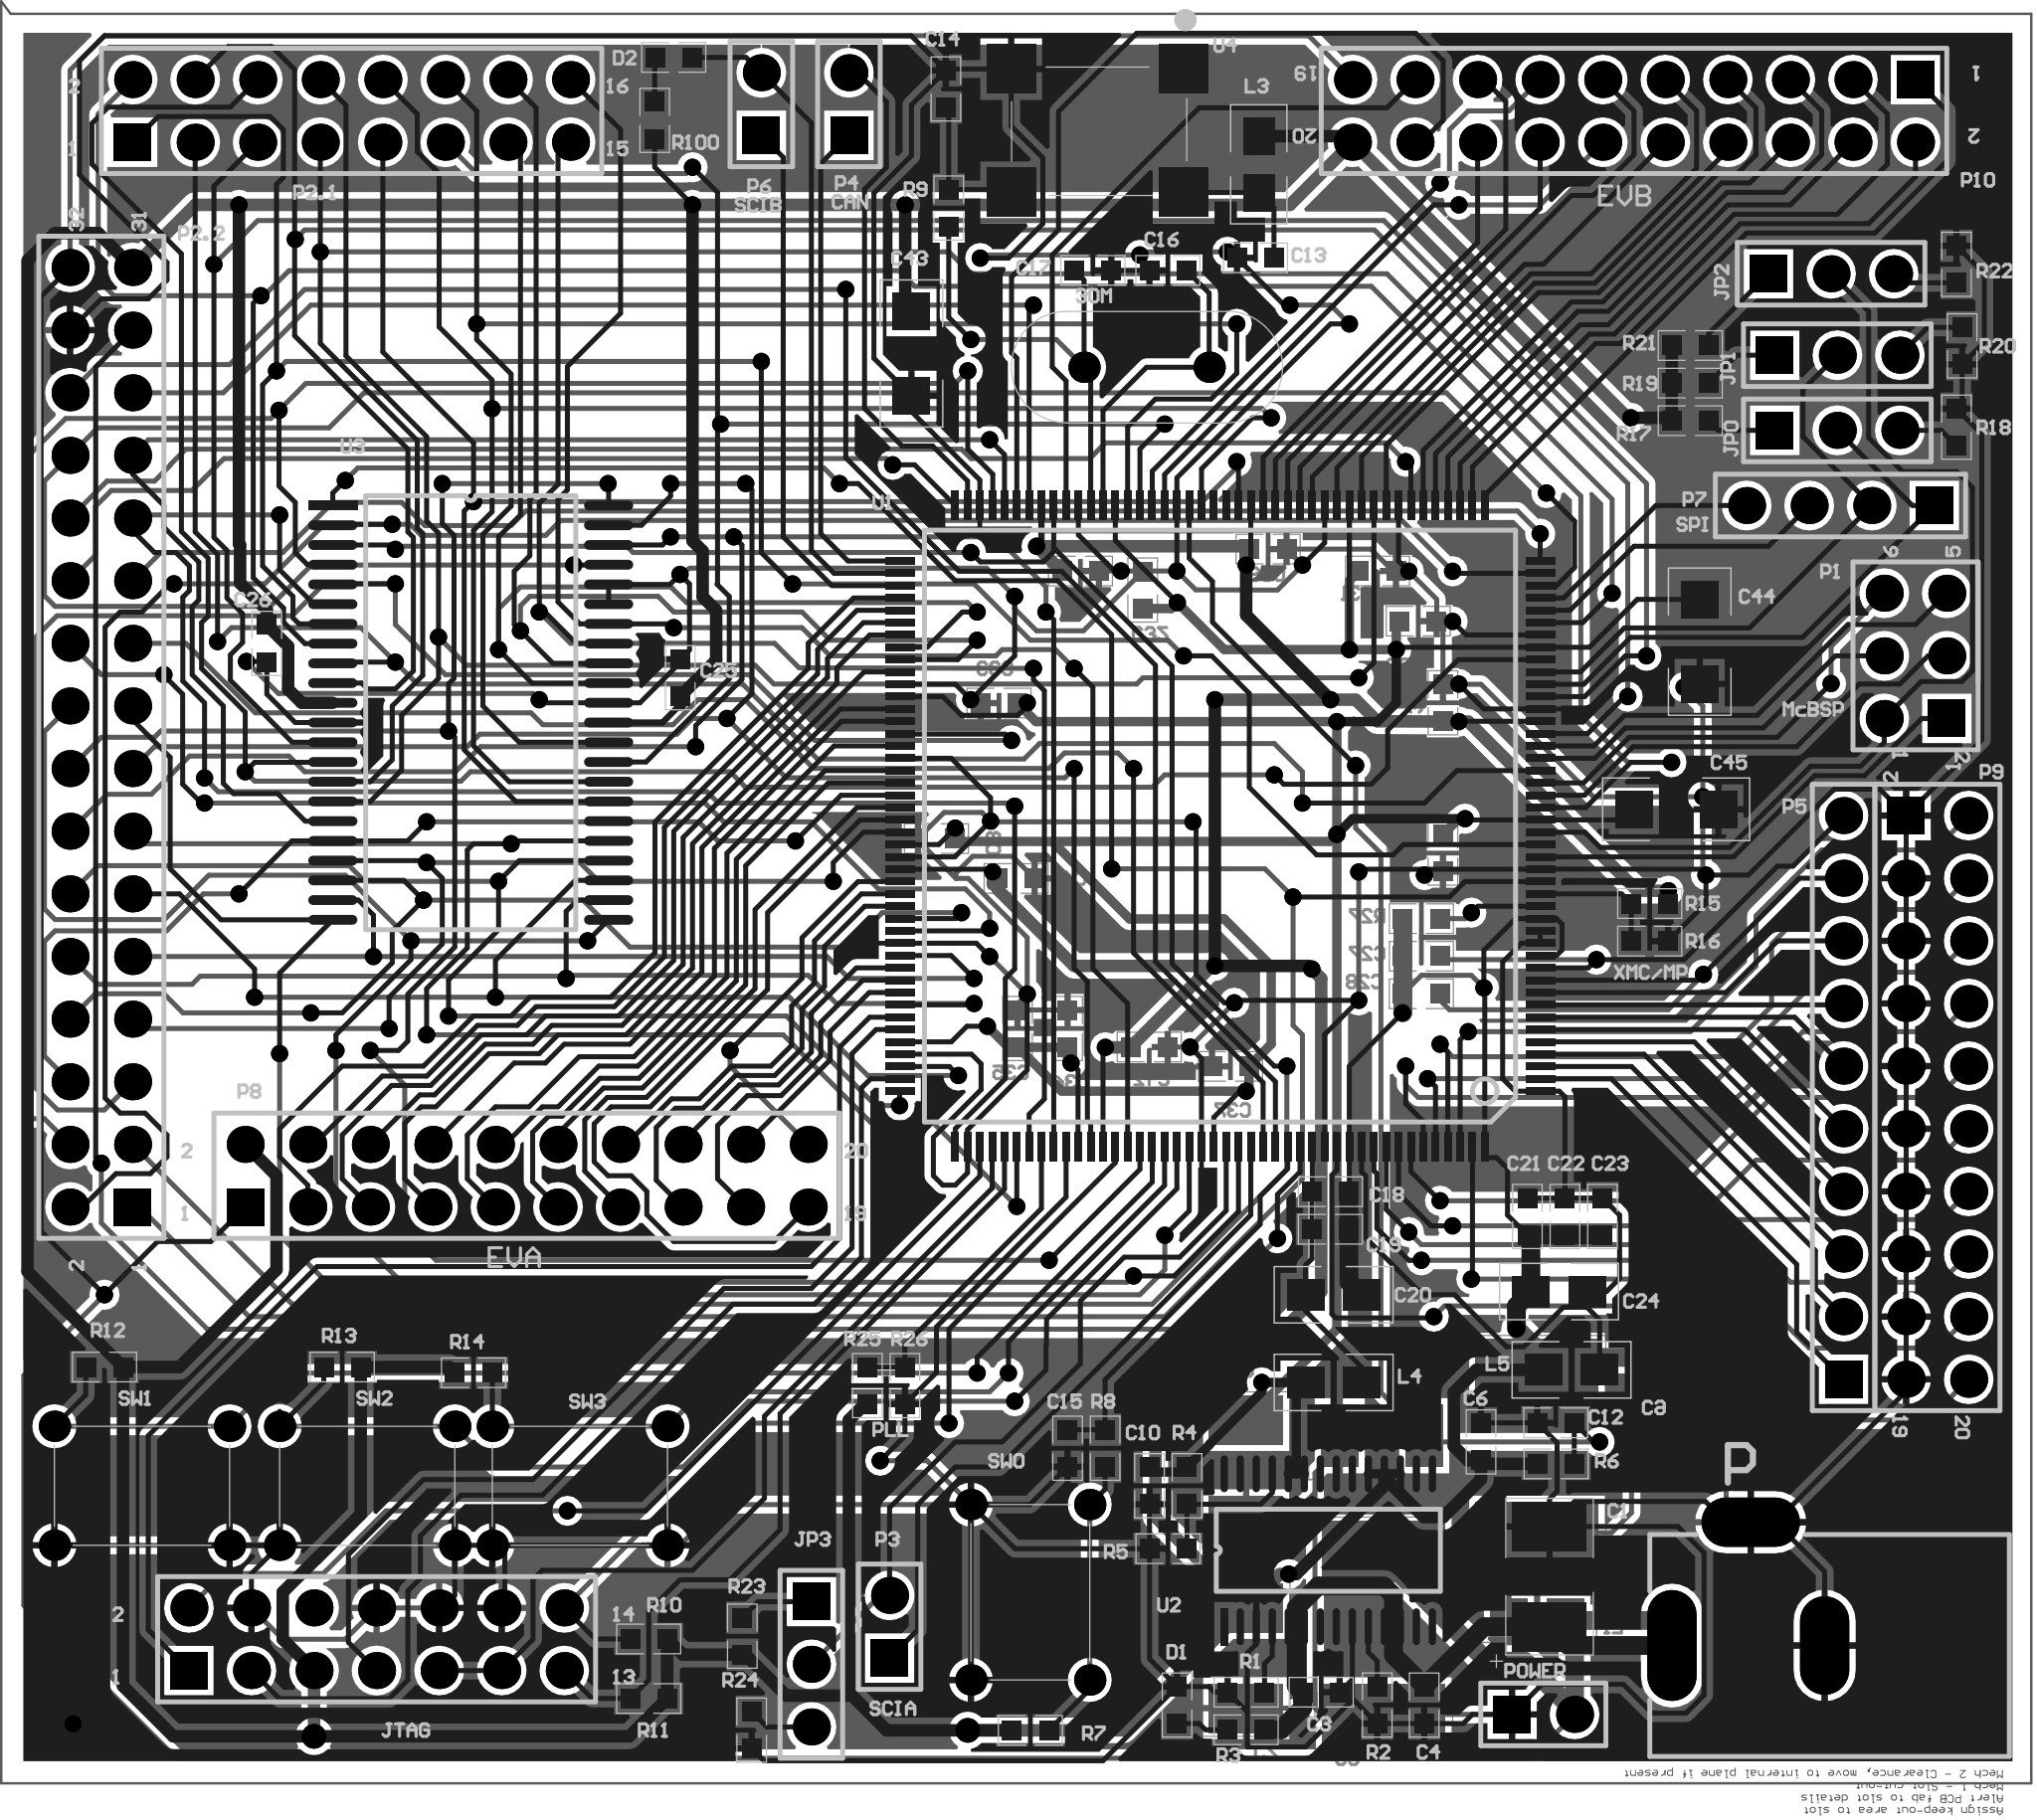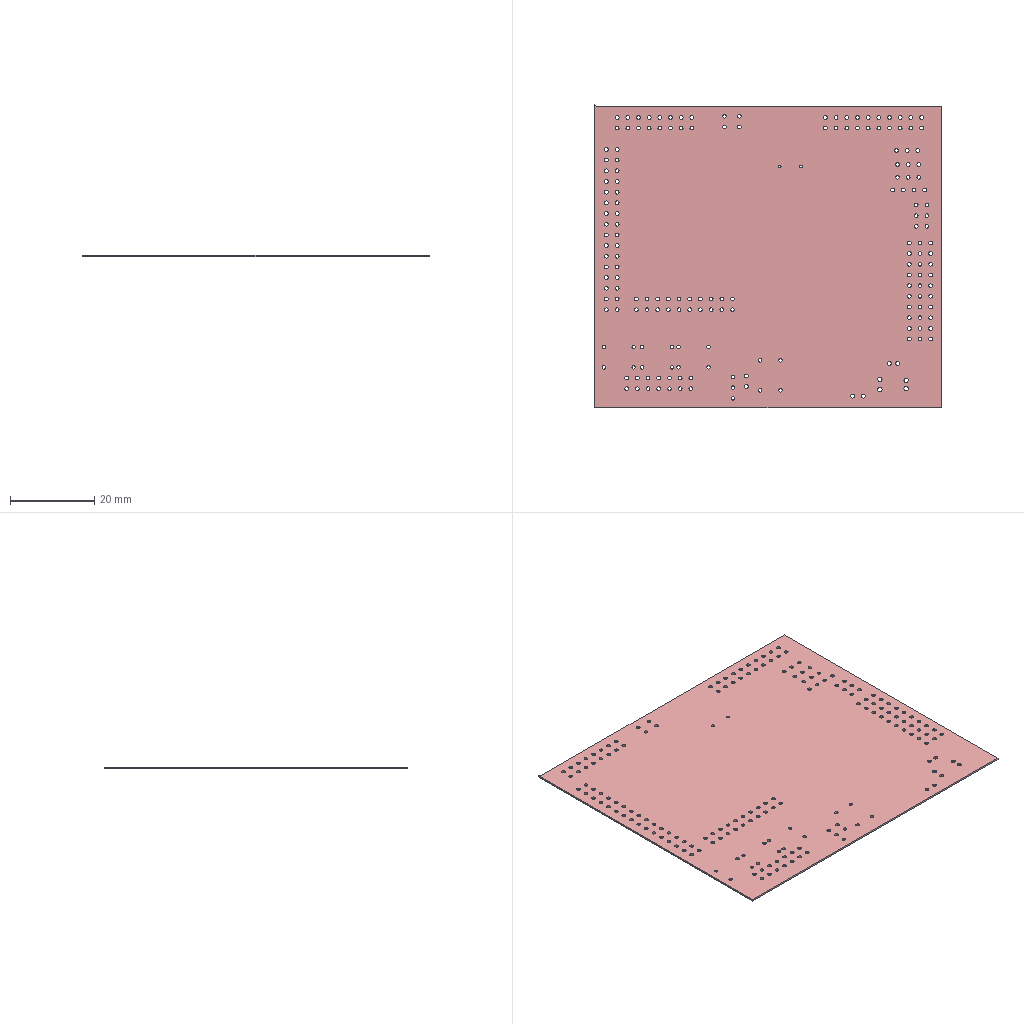Circuit board layout | Altium Designer | box 82.4 x 72.3 x 0.4 mm
Layer stack:
# Altium Designer layer stack of  (unit mm; dielectric type: 0 none, 1 core, 2 prepreg, 3 surface material)
index,name,kind,layer,copper_thickness_mm,dielectric_type,dielectric_thickness_mm,dielectric_material,dielectric_constant
0,Top Paste,other,,,,,,
1,Top Overlay,other,,,,,,
2,Top Solder,dielectric,,,3,0.0102,Solder Resist,3.5
3,Top Layer,copper,Top Layer,0.0356,,,,
4,Dielectric1,dielectric,,,0,0.32,FR-4,4.8
5,Bottom Layer,copper,Bottom Layer,0.0356,,,,
6,Bottom Solder,dielectric,,,3,0.0102,Solder Resist,3.5
7,Bottom Overlay,other,,,,,,
8,Bottom Paste,other,,,,,,
# drill layer pairs: low layer,high layer
drill_pair,Top Layer,Bottom Layer
Part placement:
Designator,Comment,Layer,Footprint,Center-X(mm),Center-Y(mm),Rotation
R100,Res2,TopLayer,0603,96.128,108.075,90
D2,RED,TopLayer,0603,96.899,110.628,0
SW2,KEY4,TopLayer,key,84.455,52.705,270
P10,Header 10X2,TopLayer,HDR2X10,135.89,108.458,180
P,PWR2.5,TopLayer,KLD-0202,140.53,48.103,180
P2.1,Header 8X2,TopLayer,HDR2X8,83.82,108.458,360
U4,30M,TopLayer,CRYSTAL1,114.102,107.656,180
U3,CY7C1041CV    SDRAM,TopLayer,TSOP44(0.8mm),88.658,84.056,360
U2,TPS767D301,TopLayer,TSOP28(0.65mm),123.478,50.09,90
U1,TMS320F2812,TopLayer,QFP176,119.08,79.457,90
SW1,KEY4,TopLayer,key,75.311,52.705,270
SW3,KEY4,TopLayer,key,93.091,52.705,270
SW0,KEY4,TopLayer,key,111.379,48.387,360
R26,2.2K,TopLayer,0603,106.288,56.767,90
R25,10k,TopLayer,0603,104.764,56.767,90
R24,2.2K,TopLayer,0603,100.065,42.797,90
R23,10k,TopLayer,0603,99.684,46.607,90
R22,2.2K,TopLayer,0603,148.982,102.237,270
R21,10k,TopLayer,0603,138.174,98.944,360
R20,2.2K,TopLayer,0603,149.214,98.931,90
R19,10K,TopLayer,0603,138.174,97.42,360
R18,2.2K,TopLayer,0603,148.982,95.633,270
R17,10K,TopLayer,0603,138.174,95.896,360
R16,1k,TopLayer,0603,136.527,74.792,180
R15,10K,TopLayer,0603,136.527,76.316,180
R14,Res2,TopLayer,0603,88.771,57.288,360
R13,Res2,TopLayer,0603,83.441,57.52,180
R12,Res2,TopLayer,0603,73.789,57.52,180
R11,Res2,TopLayer,0603,95.883,44.08,360
R10,Res2,TopLayer,0603,95.883,46.493,360
R9,1k,TopLayer,0603,108.066,104.519,90
R8,100,TopLayer,0603,114.416,54.227,90
R7,1.5K,TopLayer,0603,111.381,42.788,180
R6,Res2,TopLayer,0603,132.727,53.594,180
R5,Res2,TopLayer,0603,116.969,50.154,180
R4,Res2,TopLayer,0603,117.74,52.707,270
R3,Res2,TopLayer,0603,120.14,42.81,360
R2,Res2,TopLayer,0603,125.465,43.813,90
R1,Res2,TopLayer,0603,120.14,44.334,360
POWER,Header 2,TopLayer,HDR1X2,132.207,43.434,360
P8,Header 10X2,TopLayer,HDR2X10,90.932,65.278,360
P7,SPI,TopLayer,HDR1X4,144.272,92.456,180
P6,CAN,TopLayer,HDR1X2,100.457,108.737,90
P4,SCIB,TopLayer,HDR1X2,104.013,108.737,90
P3,SCIA,TopLayer,HDR1X2,105.664,46.99,90
P1,MCBSP,TopLayer,HDR2X3,147.32,86.36,90
L5,Inductor,TopLayer,0805,133.354,57.406,180
L3,Inductor,TopLayer,0805,120.654,106.291,90
JTAG,Header 7X2,TopLayer,HDR2X7,84.836,46.482,360
JP2,BOOT2,TopLayer,HDR1X3,143.891,101.854,360
JP1,BOOT1,TopLayer,HDR1X3,144.145,98.552,360
JP0,BOOT0,TopLayer,HDR1X3,144.145,95.504,360
D1,RED,TopLayer,0603,117.337,43.813,90
C44,Cap Pol1,TopLayer,1206,138.557,86.936,270
C43,Cap Pol1,TopLayer,1206,106.553,98.62,270
C26,Cap,TopLayer,0603,80.38,86.866,90
C25,Cap,TopLayer,0603,97.166,85.473,270
C24,Cap Pol1,TopLayer,0805,132.846,60.581,180
C23,Cap Semi,TopLayer,0603,134.609,63.625,90
C22,Cap Semi,TopLayer,0603,133.085,63.625,90
C21,Cap Semi,TopLayer,0603,131.561,63.625,90
C20,Cap Pol1,TopLayer,0805,123.694,60.45,360
C19,Cap Semi,TopLayer,0603,123.563,63.108,180
C18,Cap Semi,TopLayer,0603,123.563,64.632,180
C15,Cap,TopLayer,0603,112.892,54.227,90
C14,Cap,TopLayer,0603,107.95,109.349,270
C13,Cap,TopLayer,0603,120.521,102.5,360
C12,Cap,TopLayer,0603,132.713,55.256,360
C10,Cap,TopLayer,0603,116.216,52.707,270
C6,Cap,TopLayer,0603,129.678,54.485,270
C4,Cap,TopLayer,0603,127.37,43.813,90
C3,Cap,TopLayer,0603,123.188,44.334,360
C1,Cap Pol1,TopLayer,C2,132.461,49.022,90
30M,XTAL,TopLayer,TXAL,116.1,98.063,90
C17,Cap Semi,TopLayer,0603,113.917,101.992,360
C16,Cap Semi,TopLayer,0603,116.965,101.992,360
L4,Inductor,TopLayer,0805,123.694,56.894,360
P2.2,Header 16X2,TopLayer,HDR2X16,73.66,83.058,90
C45,Cap Pol1,TopLayer,1206,137.6,80.137,360
P9,Header 10X2,TopLayer,HDR2X10,148.209,68.453,270
P5,Header 10,TopLayer,HDR1X10,144.399,68.453,90
JP3,BOOT3,TopLayer,HDR1X3,102.489,45.466,270
R27,24.9K,BottomLayer,0603,127.256,75.703,180
L2,Inductor,BottomLayer,0805,138.942,57.91,180
L1,Inductor,BottomLayer,0805,131.957,47.496,180
C42,0.1uF,BottomLayer,0603,116.207,70.496,180
C41,0.1uF,BottomLayer,0603,110.804,77.332,360
C40,0.1uF,BottomLayer,0603,113.413,89.8,180
C39,0.1uF,BottomLayer,0603,121.033,90.689,180
C38,0.1uF,BottomLayer,0603,128.132,84.457,270
C37,0.1uF,BottomLayer,0603,119.505,69.712,360
C36,0.1uF,BottomLayer,0603,112.892,71.249,270
C35,0.1uF,BottomLayer,0603,110.86,71.249,270
C34,0.1uF,BottomLayer,0603,107.567,78.95,360
C33,0.1uF,BottomLayer,0603,110.107,84.444,360
C32,0.1uF,BottomLayer,0603,115.94,89.029,270
C31,0.1uF,BottomLayer,0603,125.475,89.8,180
C30,0.1uF,BottomLayer,0603,127.129,87.768,180
C29,0.1uF,BottomLayer,0603,128.132,78.361,270
C28,Cap,BottomLayer,0603,127.256,72.655,180
C27,Cap,BottomLayer,0603,127.256,74.179,180
C11,Cap Pol1,BottomLayer,1210,125.658,54.734,180
C9,Cap,BottomLayer,0603,137.035,54.748,180
C8,Cap Pol1,BottomLayer,C1,131.953,54.102,90
C7,Cap Pol1,BottomLayer,c2,120.142,45.72,270
C5,Cap Pol1,BottomLayer,C2,120.142,53.34,270
C2,Cap Pol1,BottomLayer,C1,125.73,46.736,270
Pad and via stacks:
# Altium Designer via and pad stacks of  (unit mm). Each distinct definition once, with the count of objects using it.
# via: kind,start_layer,end_layer,hole_mm,diameter_mm,mode(0 simple;1 top-mid-bottom;2 full stack),diameter_per_layer,count,example_net
# pad: kind,layer,hole_mm,hole_type(0 round;1 square;2 slot),plating,top_size,top_shape(1 round;2 rect;3 octagon;9 rounded rect),mid_size,bottom_size,mode,footprint,size_per_layer,count,example
pad,Top Layer,0,0,plated,0.8x0.8,2,0.8x0.8,0.8x0.8,0,0603,,92,D2.2
pad,Top Layer,0,0,plated,1.524x1.524,2,1.524x1.524,1.524x1.524,0,1206,,6,C45.1
pad,Top Layer,0,0,plated,2x0.4,1,2x0.4,2x0.4,0,TSOP44(0.8mm),,43,U3.6
pad,Top Layer,0,0,plated,1.2x0.3,2,1.2x0.3,1.2x0.3,0,QFP176,,176,U1.133
pad,Top Layer,0,0,plated,2x2,2,2x2,2x2,0,CRYSTAL1,,4,U4.4
pad,Top Layer,0,0,plated,1.524x1.27,2,1.524x1.27,1.524x1.27,0,0805,,10,L3.1
pad,Top Layer,0,0,plated,2x0.4,2,2x0.4,2x0.4,0,TSOP44(0.8mm),,1,U3.1
pad,Top Layer,0,0,plated,1.5x0.3,2,1.5x0.3,1.5x0.3,0,TSOP28(0.65mm),,1,U2.1
pad,Top Layer,0,0,plated,1.5x0.3,1,1.5x0.3,1.5x0.3,0,TSOP28(0.65mm),,27,U2.2
pad,Top Layer,0,0,plated,2x3,2,2x3,2x3,0,C2,,2,C1.2
pad,Bottom Layer,0,0,plated,1.524x2.54,2,1.524x2.54,1.524x2.54,0,1210,,2,C11.2
pad,Bottom Layer,0,0,plated,2x3,2,2x3,2x3,0,c2,,4,C7.2
pad,Bottom Layer,0,0,plated,2.5x5,2,2.5x5,2.5x5,0,C1,,4,C2.1
pad,Bottom Layer,0,0,plated,0.8x0.8,2,0.8x0.8,0.8x0.8,0,0603,,36,C9.1
pad,Bottom Layer,0,0,plated,1.524x1.27,2,1.524x1.27,1.524x1.27,0,0805,,4,L2.2
pad,Multi-Layer,0.8128,0,plated,1.27x1.27,1,1.27x1.27,1.27x1.27,0,key,,16,SW2.3
pad,Multi-Layer,0.9,0,plated,1.5x1.5,1,1.5x1.5,1.5x1.5,0,HDR2X10,,57,P10.20
pad,Multi-Layer,0.9,0,plated,1.5x1.5,2,1.5x1.5,1.5x1.5,0,HDR2X10,,3,P10.1
pad,Multi-Layer,1,0,plated,1.5x1.5,1,1.5x1.5,1.5x1.5,0,KLD-0202,,6,P.1A
pad,Multi-Layer,0,0,plated,4x2,1,4x2,4x2,0,KLD-0202,,1,P.3
pad,Multi-Layer,0,0,plated,2x4,1,2x4,2x4,0,KLD-0202,,1,P.2
pad,Multi-Layer,0,0,plated,2x4.5,1,2x4.5,2x4.5,0,KLD-0202,,1,P.1
pad,Multi-Layer,0.9,0,plated,1.5x1.5,1,1.5x1.5,1.5x1.5,0,HDR2X8,,15,P2.1.16
pad,Multi-Layer,0.9,0,plated,1.5x1.5,2,1.5x1.5,1.5x1.5,0,HDR2X8,,1,P2.1.1
pad,Multi-Layer,0.9,0,plated,1.5x1.5,2,1.5x1.5,1.5x1.5,0,HDR1X3,,4,JP0.1
pad,Multi-Layer,0.9,0,plated,1.5x1.5,1,1.5x1.5,1.5x1.5,0,HDR1X3,,8,JP0.2
pad,Multi-Layer,0.9,0,plated,1.5x1.5,1,1.5x1.5,1.5x1.5,0,HDR2X7,,13,JTAG.14
pad,Multi-Layer,0.9,0,plated,1.5x1.5,2,1.5x1.5,1.5x1.5,0,HDR2X7,,1,JTAG.1
pad,Multi-Layer,0.9,0,plated,1.5x1.5,1,1.5x1.5,1.5x1.5,0,HDR1X2,,4,P4.2
pad,Multi-Layer,0.9,0,plated,1.5x1.5,2,1.5x1.5,1.5x1.5,0,HDR1X2,,4,P4.1
pad,Multi-Layer,0.9,0,plated,1.5x1.5,1,1.5x1.5,1.5x1.5,0,HDR2X3,,5,P1.6
pad,Multi-Layer,0.9,0,plated,1.5x1.5,2,1.5x1.5,1.5x1.5,0,HDR2X3,,1,P1.1
pad,Multi-Layer,0.9,0,plated,1.5x1.5,1,1.5x1.5,1.5x1.5,0,HDR1X4,,3,P7.4
pad,Multi-Layer,0.9,0,plated,1.5x1.5,2,1.5x1.5,1.5x1.5,0,HDR1X4,,1,P7.1
pad,Multi-Layer,0.7,0,plated,1.27x1.27,1,1.27x1.27,1.27x1.27,0,TXAL,,2,30M.1
pad,Multi-Layer,0.9,0,plated,1.5x1.5,1,1.5x1.5,1.5x1.5,0,HDR2X16,,31,P2.2.32
pad,Multi-Layer,0.9,0,plated,1.5x1.5,2,1.5x1.5,1.5x1.5,0,HDR2X16,,1,P2.2.1
pad,Multi-Layer,0.9,0,plated,1.5x1.5,2,1.5x1.5,1.5x1.5,0,HDR1X10,,1,P5.1
pad,Multi-Layer,0.9,0,plated,1.5x1.5,1,1.5x1.5,1.5x1.5,0,HDR1X10,,9,P5.2
via,Top Layer,Bottom Layer,0.3,0.7,0,,194,GND
via,Top Layer,Bottom Layer,0.5,1,0,,2,3.3V
Copper pours:
name,layer,net,type(0 solid;1 hatched;2 none)
Top Layer-GND,Top Layer,GND,0
Bottom Layer-GND,Bottom Layer,GND,0
Design rules, without the lines most boards share:
# Altium Designer design rules of  (exported by Altium Designer, unit mm)
# columns: name | kind | enabled | priority | scope1 | scope2 | descriptor | typed fields (field=value)
HoleToHoleClearance | 52 | enabled | 1 | All | All | Hole To Hole Clearance (Gap=10mil) (All),(All) | gap=0.254
DiffPairsRouting | 51 | enabled | 1 | All | All | Differential Pairs Uncoupled Length using the Gap Constraints (Min=10mil) (Max=10mil) (Prefered=10mil)  and Width Constraints (Min=15mil) (Max=15mil) (Prefered=15mil) (All) |
Clearance | 0 | enabled | 1 | All | All | Clearance Constraint (Gap=7mil) (All),(All) | gap=0.1778
PlaneConnect | 6 | enabled | 1 | All | All | Power Plane Connect Rule(Relief Connect )(Expansion=20mil) (Conductor Width=10mil) (Air Gap=10mil) (Entries=4) (All) | relief_conductor_width=0.254 relief_entries=4 relief_expansion=0.508
PolygonConnect | 20 | enabled | 1 | All | All | Polygon Connect Rule(Relief Connect )(Conductor Width=10mil) (Relief Angle=90 Angle) (Entries=4) (Air Gap Width=10mil) (All),(All) | connect_style(0=relief,1=direct,2=none)=0 relief_conductor_width=0.254 relief_entries=4
Width | 2 | enabled | 3 | All | All | Width Constraint (Min=8mil) (Max=39.37mil) (Preferred=8mil) (All) |
RoutingVias | 11 | enabled | 1 | All | All | Routing Via (MinHoleWidth=11mil) (MaxHoleWidth=39.37mil) (PreferredHoleWidth=11.811mil) (MinWidth=27mil) (MaxWidth=39.37mil) (PreferedWidth=27.559mil) (All) | via_min_hole=0.2794 via_max_hole=1 via_preferred_diameter=0.7 via_preferred_hole=0.3
SolderMaskExpansion | 13 | enabled | 1 | All | All | Solder Mask Expansion (Expansion =4mil) (All) | expansion=0.1016
TestPointUsage | 44 | enabled | 1 | All | All | Fabrication Testpoint Usage (Valid =One Required, Allow multiple per net=No) (All) |
Testpoint | 43 | enabled | 1 | All | All | Fabrication Testpoint Style (Under Component=Yes) (All) |
Width_1 | 2 | enabled | 2 | InNet('1.8V') | All | Width Constraint (Min=8mil) (Max=30mil) (Preferred=15mil) (InNet('1.8V')) |
Width_2 | 2 | enabled | 1 | InNet('3.3V') | All | Width Constraint (Min=8mil) (Max=30mil) (Preferred=20mil) (InNet('3.3V')) |
Classes set for this board:
# Altium Designer classes of  (member kind: 0 net, 1 component, 2 from-to, 3 pad, 4 layer, 5 differential pair, 6 design channel, 7 polygon, 8 structure, 9 xSignal)
# columns: class name | member kind | superclass | members
2812 | 1 | no | *; 30M; C1; C2; C3; C4; C5; C6; C7; C8; C9; C10; C11; C12; C13; C14; C15; C16; C17; C18; C19; C20; C21; C22; C23; C24; C25; C26; C27; C28; C29; C30; C31; C32; C33; C34; C35; C36; C37; C38; C39; C40; C41; C42; C43; C44; C45; D1; JP2; JP0; JP1; JP2; JP2; JTAG; L1; L2; L3; L4; L5; C33; P1; P3; P4; P5; P6; P7; P8; P9; POWER; R1; R2; R3; R4; R5; R6; R7; R8; R9; R10; R11; R12; R13; R14; R15; R16; R17; R18; R19; R20; R21; R22; R23; R24; R25; R26; R27; SW0; SW0; SW0; SW1; U1; U2; U3; D1; 30M; C1; C2; C3; C4; C5; C6; C7; C8; C9; C10; C11; C12; C13; C14; C15; C16; C17; C18; C19; C20; C21; C22; C23; C24; C25; C26; C27; C28; C29; C30; C31; C32; C33; C34; C35; C36; C37; C38; C39; C40; C41; C42; C43; C44; C45; D1; JP2; JP0; JP1; JP2; JP2; JTAG; L1; L2; L3; L4; L5; P1; P3; P4; P5; P6; P7; P8; P9; POWER; C33; R1; R2; R3; R4; R5; R6; R7; R8; R9; R10; R11; R12; R13; R14; R15; R16; R17; R18; R19; R20; R21; R22; R23; R24; R25; R26; R27; SW0; SW0; SW0; SW1; U1; U2; U3; 30M; C1; C2; C3; C4; C5; C6; C7; C8; C9; C10; C11; C12; C13; C14; C15; C16; C17; C18; C19; C20; C21; C22; C23; C24; C25; C26; C27; C28; C29; C30; C31; C32; C33; C34; C35; C36; C37; C38; C39; C40; C41; C42; C43; C44; C45; D1; JP2; JP0; JP1; JP2; JP2; JTAG; L1; L2; L3; L4; L5; P1; P3; P4; P5; P6; P7; P8; P9; POWER; C33; R1; R2; R3; R4; R5; R6; R7; R8; R9; R10; R11; R12; R13; R14; R15; R16; R17; R18; R19; R20; R21; R22; R23; R24; R25; R26; R27; SW0; SW0; SW0; SW1; U1; U2; U3; U4; P10; SW1; SW2; JP3; JP4; P2.1; P2.2; P2.2; C33; SW1; D2; P; R100; SW3;